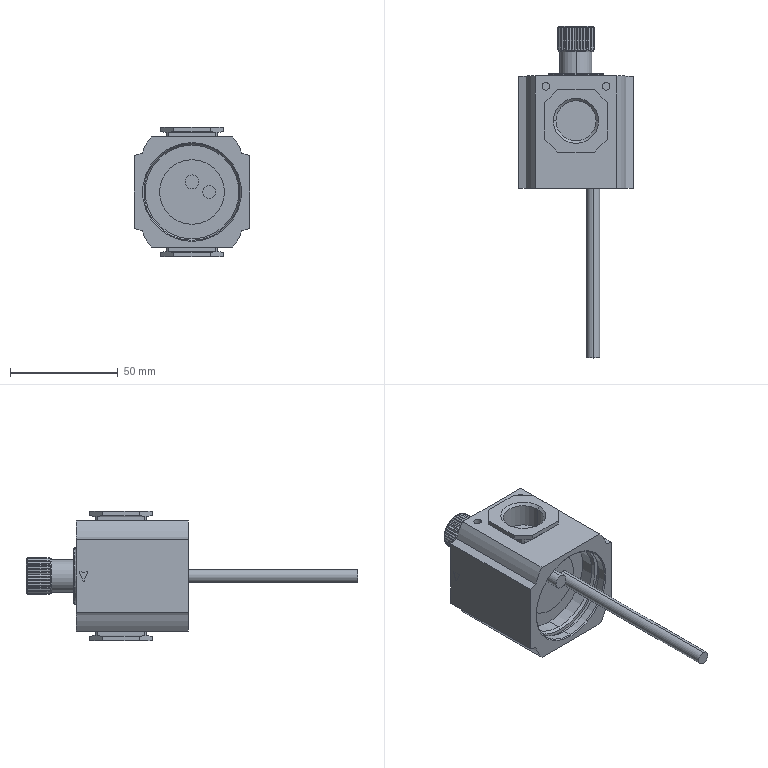Part | STEP file | Copy 19^GFC30015-A-F1 | 1 solid | 418 faces | box 53.5 x 153.9 x 60 mm | volume 118131 mm3 | plane 295 | cylinder 107 | cone 10 | spline 6 | commonest cylinder face diameters 0.4 x9 0.8 x8 3.5 x8 0.9 x7 1.6 x7 6 x7